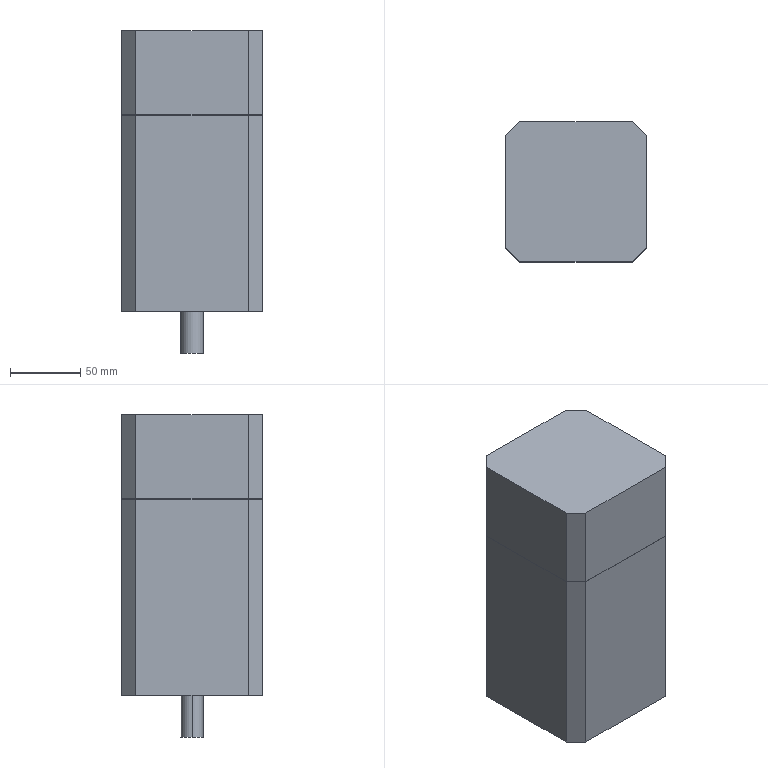Part | STEP file | Servo | 2 solids | 26 faces | box 100 x 100 x 230 mm | volume 1946815 mm3 | plane 22 | cylinder 4 | commonest cylinder face diameters 16 x2 70 x2